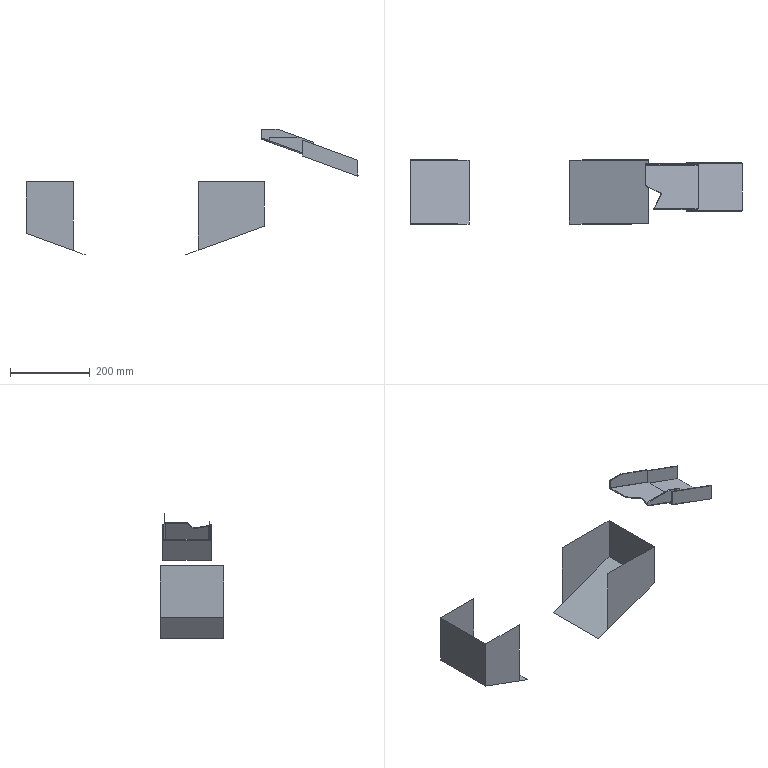Part | CATIA | 2 solids | 60 faces | box 830.623 x 160 x 315 mm | volume 5795629 mm3 | plane 45 | spline 11 | cylinder 4 | commonest cylinder face diameters 2 x2 6 x2